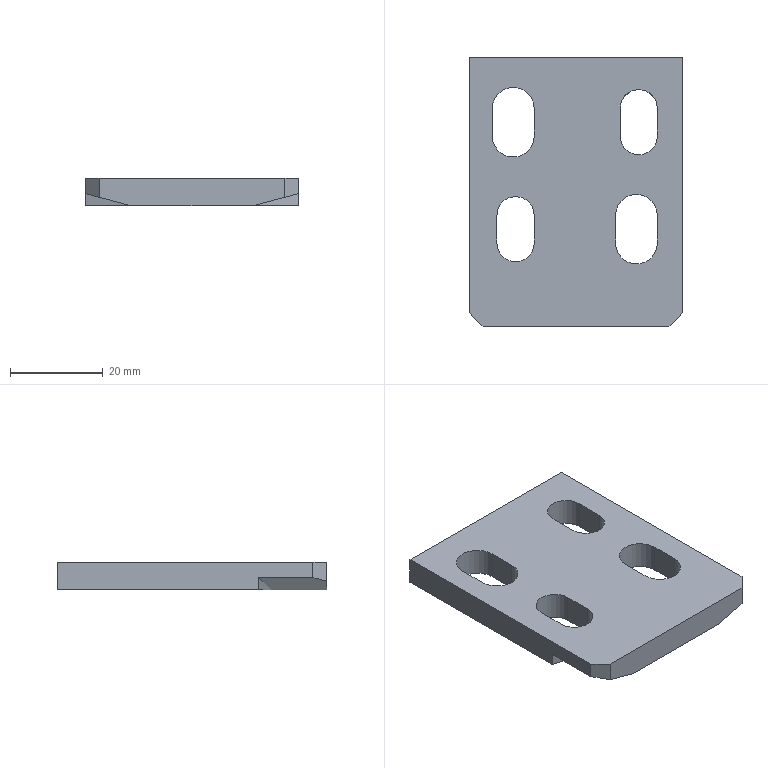Part | STEP file | gslz 2016.10.28-13_id678_x_t | 1 solid | 28 faces | box 46 x 58 x 6 mm | volume 13016 mm3 | plane 20 | cylinder 8 | commonest cylinder face diameters 8 x4 9 x4